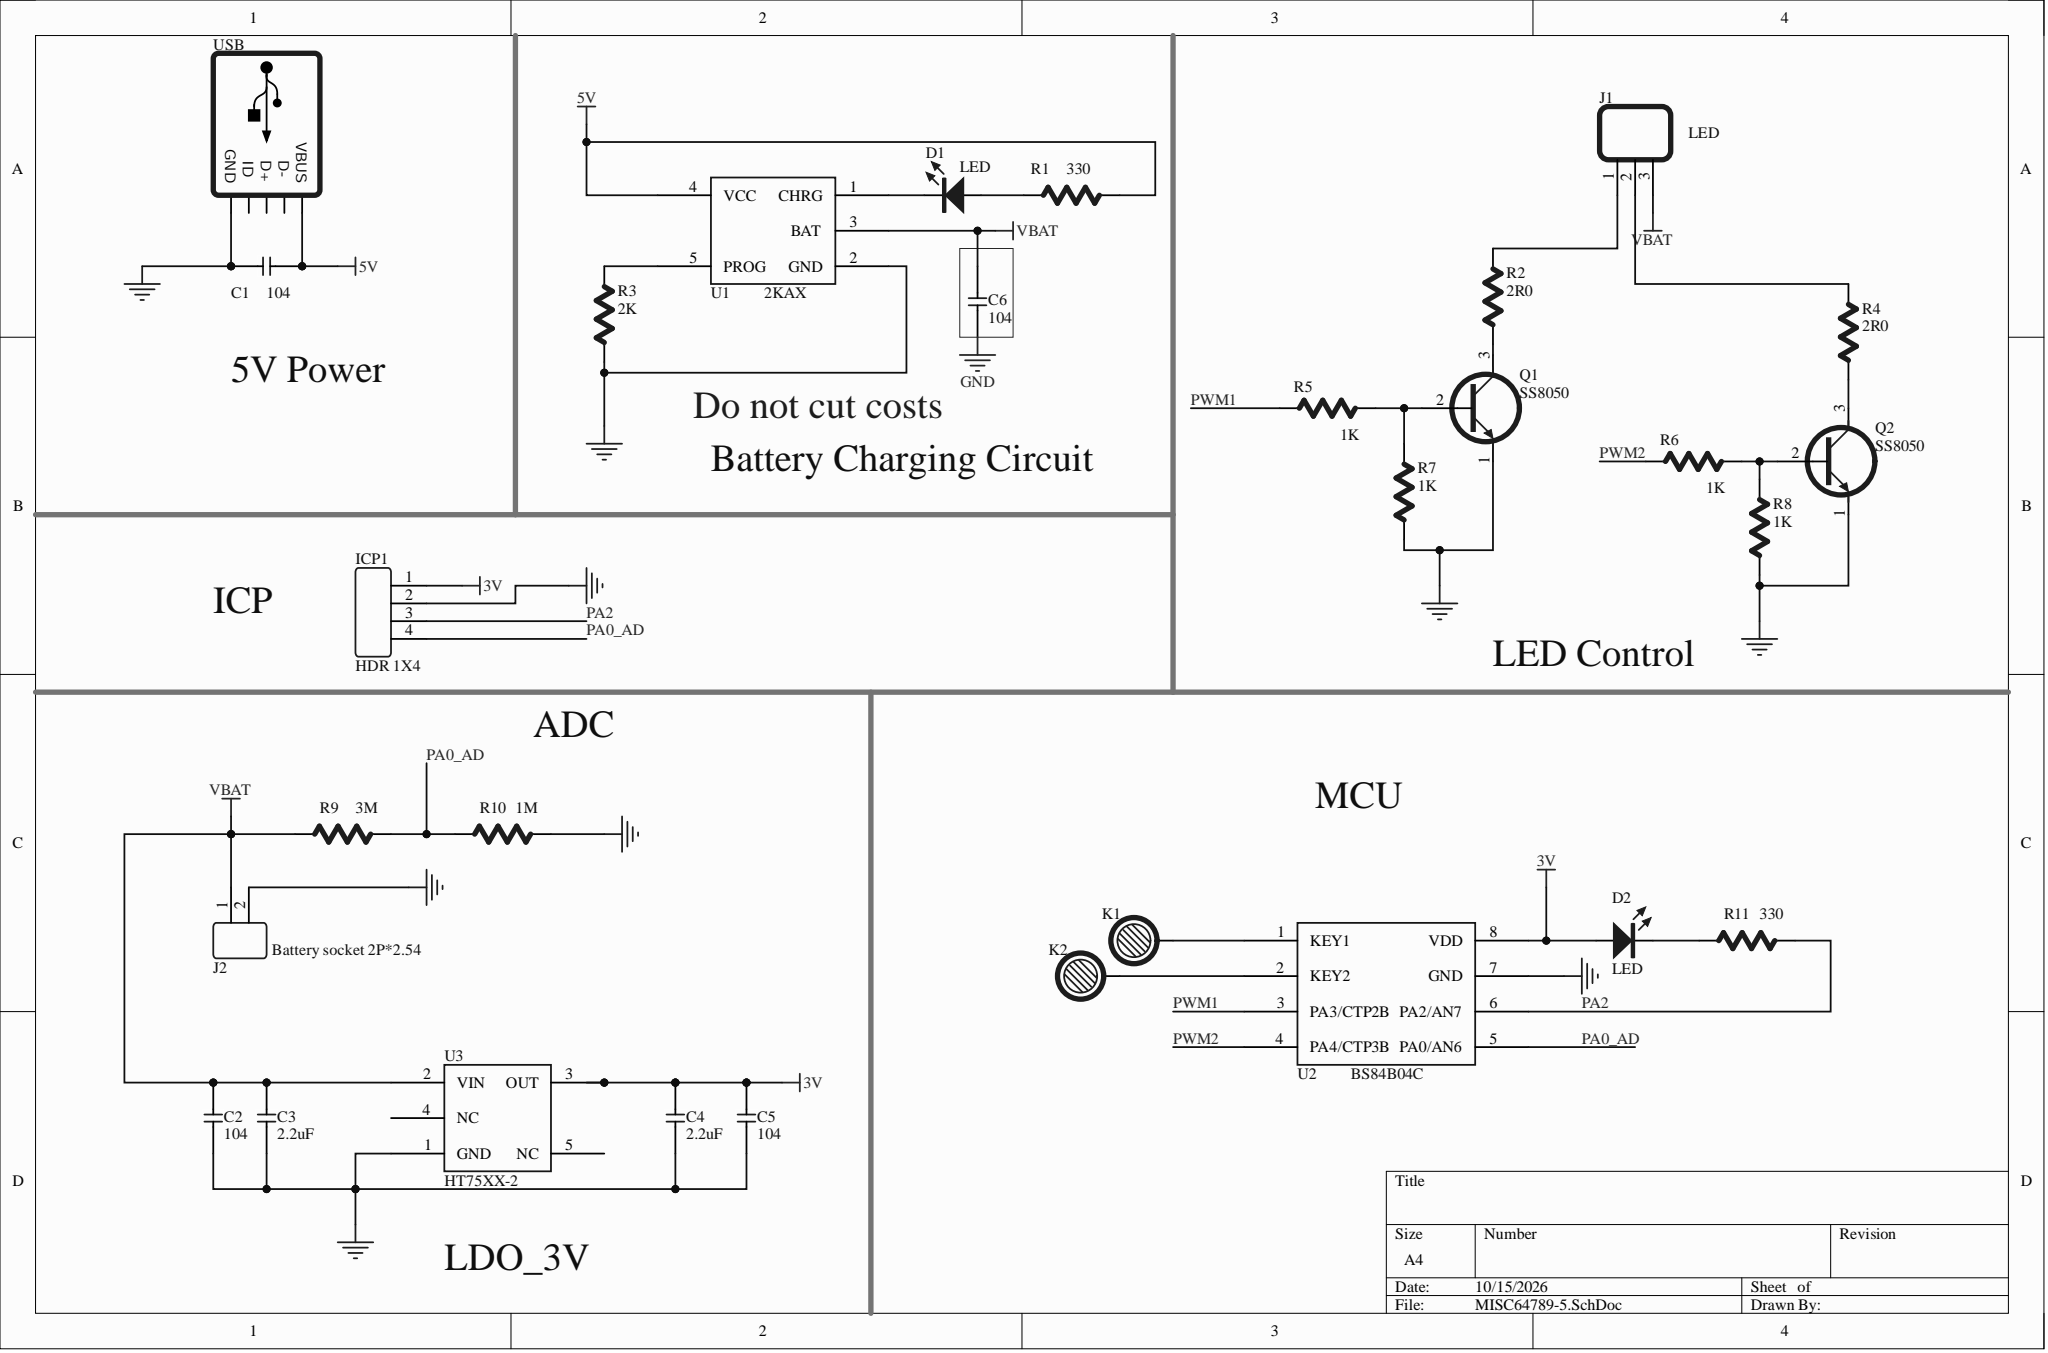Circuit board | Altium Designer | 30 parts | 20 nets
Bill of materials:
Comment,Description,Designator,Footprint,LibRef,Quantity
"104","?, [NoValue]","C1, C2, C5, C6","C 0603","Cap","4"
"2.2uF","[NoValue], ?","C3, C4","C 0603","Cap","2"
"LED","Typical INFRARED GaAs LED","D1, D2","LED_0603","LED(1)","2"
"HDR 1X4","","ICP1","HDR 1x4(2.54)","HDR 1X4(?)","1"
"LED","","J1","HDR1X3","HDR 1X3_2","1"
"Battery socket 2P*2.54","","J2","HDR 1X2 Pitch 2.5mm","HDR 1X2(?)","1"
"TOUCHKEY","","K1, K2","KEY","Touch Pad(1)","2"
"SS8050","NPN Bipolar Transistor","Q1, Q2","SOT23_BJT_NPN","BJT_NPN","2"
"330","Resisitor","R1, R11","R 0603","Resistor(1)","2"
"2R0","Resisitor","R2, R4","R 1206","Resistor(1)","2"
"2K","Resisitor","R3","R 0603","Resistor(1)","1"
"1K","Resisitor","R5, R6, R7, R8","R 0603","Resistor(1)","4"
"3M","Resisitor","R9","R 0603","Resistor(1)","1"
"1M","Resisitor","R10","R 0603","Resistor(1)","1"
"2KAX","","U1","SOT23 PIN-5","2KAX","1"
"BS84B04C","","U2","SOP8","BS84B04C","1"
"HT75XX-2","","U3","SOT23 PIN-5","HT7530","1"
"USB","Mini/Micro","USB","Micro USB_02","USB(2_1)","1"
Netlist (Protel format):
[
C1
C 0603
104



]
[
C2
C 0603
104



]
[
C3
C 0603
2.2uF



]
[
C4
C 0603
2.2uF



]
[
C5
C 0603
104



]
[
C6
C 0603
104



]
[
D1
LED_0603
LED



]
[
D2
LED_0603
LED



]
[
ICP1
HDR 1x4(2.54)
HDR 1X4



]
[
J1
HDR1X3
LED



]
[
J2
HDR 1X2 Pitch 2.5mm
Battery socket 2P*2.54



]
[
K1
KEY
TOUCHKEY



]
[
K2
KEY
TOUCHKEY



]
[
Q1
SOT23_BJT_NPN
SS8050



]
[
Q2
SOT23_BJT_NPN
SS8050



]
[
R1
R 0603
330



]
[
R2
R 1206
2R0



]
[
R3
R 0603
2K



]
[
R4
R 1206
2R0



]
[
R5
R 0603
1K



]
[
R6
R 0603
1K



]
[
R7
R 0603
1K



]
[
R8
R 0603
1K



]
[
R9
R 0603
3M



]
[
R10
R 0603
1M



]
[
R11
R 0603
330



]
[
U1
SOT23 PIN-5
2KAX



]
[
U2
SOP8
BS84B04C



]
[
U3
SOT23 PIN-5
HT75XX-2



]
[
USB
Micro USB_02
USB



]
(
VBAT
C2-2
C3-2
C6-1
J1-3
J2-1
R9-1
U1-3
U3-2
)
(
PWM2
R6-1
U2-4
)
(
PWM1
R5-1
U2-3
)
(
PA2
ICP1-3
R11-2
U2-6
)
(
PA0_AD
ICP1-4
R9-2
R10-1
U2-5
)
(
NetR3_2
R3-2
U1-5
)
(
NetQ2_3
Q2-3
R4-1
)
(
NetQ2_2
Q2-2
R6-2
R8-2
)
(
NetQ1_3
Q1-3
R2-1
)
(
NetQ1_2
Q1-2
R5-2
R7-2
)
(
NetK2_1
K2-1
U2-2
)
(
NetK1_1
K1-1
U2-1
)
(
NetJ1_2
J1-2
R4-2
)
(
NetJ1_1
J1-1
R2-2
)
(
NetD2_2
D2-2
R11-1
)
(
NetD1_2
D1-2
U1-1
)
(
NetD1_1
D1-1
R1-1
)
(
GND
C1-2
C2-1
C3-1
C4-1
C5-1
C6-2
ICP1-2
J2-2
Q1-1
Q2-1
R3-1
R7-1
R8-1
R10-2
U1-2
U2-7
U3-1
USB-5
)
(
5V
C1-1
R1-2
U1-4
USB-1
)
(
3V
C4-2
C5-2
D2-1
ICP1-1
U2-8
U3-3
)